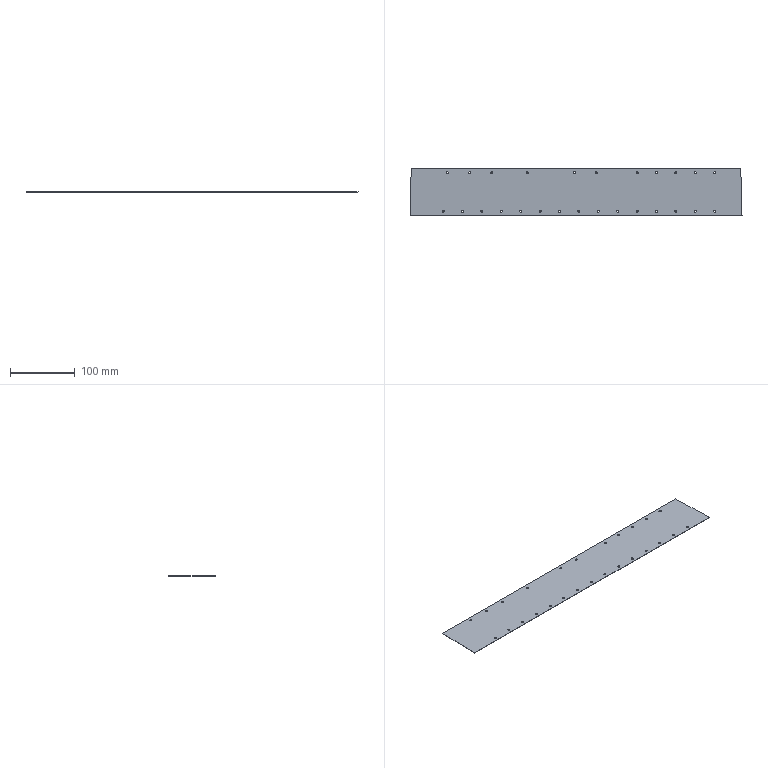Part | SolidWorks | features BaseBody 1 | 1 solid | 58 faces | box 513.4 x 71.5 x 0.5 mm | volume 18183 mm3 | cylinder 52 | plane 6 | commonest cylinder face diameters 3.2 x52